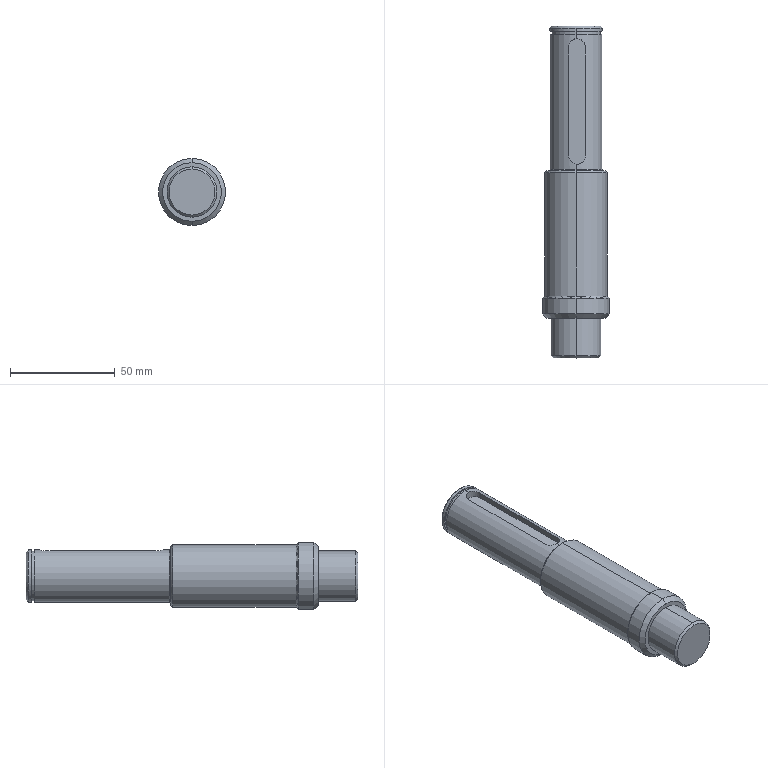Part | SolidWorks | features BaseBody 1 | 1 solid | 42 faces | box 32 x 158.5 x 32 mm | volume 90096 mm3 | cylinder 16 | cone 12 | plane 10 | spline 4 | commonest cylinder face diameters 25 x4 6.647 x2 8 x2 23.5 x2 24 x2 30 x2